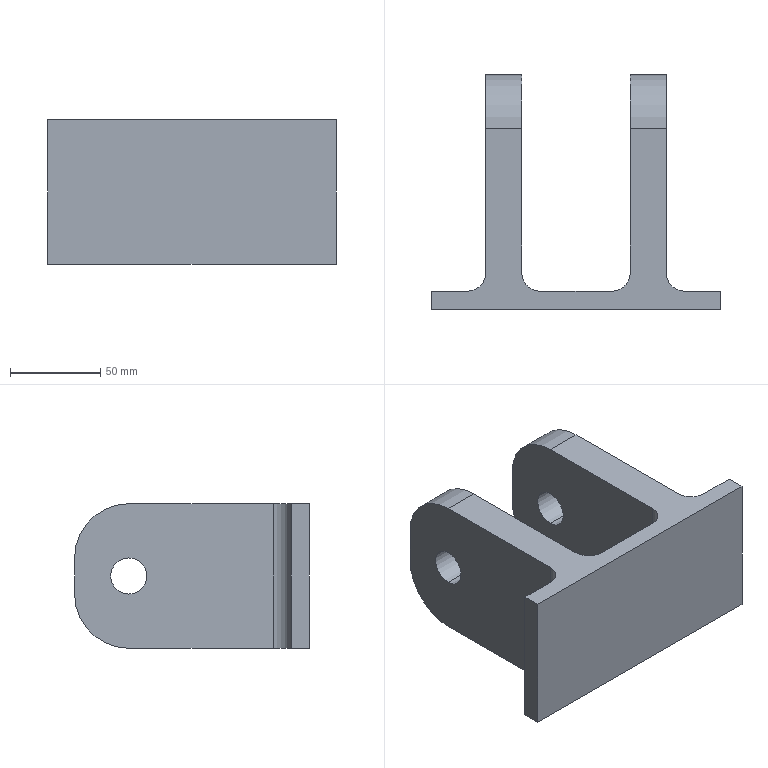Part | STEP file | Hydraulic cylinder base | 1 solid | 26 faces | box 160 x 130 x 80 mm | volume 490850 mm3 | plane 14 | cylinder 12 | commonest cylinder face diameters 20 x8 60 x4
STEP:
#1=CARTESIAN_POINT('',(50.,100.,10.));
#2=VERTEX_POINT('',#1);
#3=CARTESIAN_POINT('',(50.,100.,-10.));
#4=VERTEX_POINT('',#3);
#5=CARTESIAN_POINT('',(50.,100.,0.));
#6=DIRECTION('',(1.,0.,0.));
#7=DIRECTION('',(0.,0.,-1.));
#8=AXIS2_PLACEMENT_3D('',#5,#6,#7);
#9=CIRCLE('',#8,10.);
#10=EDGE_CURVE('',#2,#4,#9,.T.);
#11=ORIENTED_EDGE('',*,*,#10,.T.);
#12=CARTESIAN_POINT('',(30.,100.,-10.));
#13=VERTEX_POINT('',#12);
#14=CARTESIAN_POINT('',(80.001,100.,-10.));
#15=DIRECTION('',(-1.,0.,0.));
#16=VECTOR('',#15,1000.);
#17=LINE('',#14,#16);
#18=EDGE_CURVE('',#4,#13,#17,.T.);
#19=ORIENTED_EDGE('',*,*,#18,.T.);
#20=CARTESIAN_POINT('',(30.,100.,10.));
#21=VERTEX_POINT('',#20);
#22=CARTESIAN_POINT('',(30.,100.,0.));
#23=DIRECTION('',(1.,0.,0.));
#24=DIRECTION('',(0.,0.,-1.));
#25=AXIS2_PLACEMENT_3D('',#22,#23,#24);
#26=CIRCLE('',#25,10.);
#27=EDGE_CURVE('',#21,#13,#26,.T.);
#28=ORIENTED_EDGE('',*,*,#27,.F.);
#29=CARTESIAN_POINT('',(80.001,100.,10.));
#30=DIRECTION('',(-1.,0.,0.));
#31=VECTOR('',#30,1000.);
#32=LINE('',#29,#31);
#33=EDGE_CURVE('',#2,#21,#32,.T.);
#34=ORIENTED_EDGE('',*,*,#33,.F.);
#35=EDGE_LOOP('',(#11,#19,#28,#34));
#36=FACE_OUTER_BOUND('',#35,.T.);
#37=CARTESIAN_POINT('',(80.001,100.,0.));
#38=DIRECTION('',(-1.,0.,0.));
#39=DIRECTION('',(0.,0.,1.));
#40=AXIS2_PLACEMENT_3D('',#37,#38,#39);
#41=CYLINDRICAL_SURFACE('',#40,10.);
#42=ADVANCED_FACE('',(#36),#41,.F.);
#43=CARTESIAN_POINT('',(-50.,100.,-10.));
#44=VERTEX_POINT('',#43);
#45=CARTESIAN_POINT('',(-50.,100.,10.));
#46=VERTEX_POINT('',#45);
#47=CARTESIAN_POINT('',(-50.,100.,0.));
#48=DIRECTION('',(-1.,0.,0.));
#49=DIRECTION('',(0.,0.,-1.));
#50=AXIS2_PLACEMENT_3D('',#47,#48,#49);
#51=CIRCLE('',#50,10.);
#52=EDGE_CURVE('',#44,#46,#51,.T.);
#53=ORIENTED_EDGE('',*,*,#52,.T.);
#54=CARTESIAN_POINT('',(-30.,100.,10.));
#55=VERTEX_POINT('',#54);
#56=CARTESIAN_POINT('',(-80.001,100.,10.));
#57=DIRECTION('',(1.,0.,0.));
#58=VECTOR('',#57,1000.);
#59=LINE('',#56,#58);
#60=EDGE_CURVE('',#46,#55,#59,.T.);
#61=ORIENTED_EDGE('',*,*,#60,.T.);
#62=CARTESIAN_POINT('',(-30.,100.,-10.));
#63=VERTEX_POINT('',#62);
#64=CARTESIAN_POINT('',(-30.,100.,0.));
#65=DIRECTION('',(1.,0.,0.));
#66=DIRECTION('',(0.,0.,-1.));
#67=AXIS2_PLACEMENT_3D('',#64,#65,#66);
#68=CIRCLE('',#67,10.);
#69=EDGE_CURVE('',#55,#63,#68,.T.);
#70=ORIENTED_EDGE('',*,*,#69,.T.);
#71=CARTESIAN_POINT('',(-80.001,100.,-10.));
#72=DIRECTION('',(1.,0.,0.));
#73=VECTOR('',#72,1000.);
#74=LINE('',#71,#73);
#75=EDGE_CURVE('',#44,#63,#74,.T.);
#76=ORIENTED_EDGE('',*,*,#75,.F.);
#77=EDGE_LOOP('',(#53,#61,#70,#76));
#78=FACE_OUTER_BOUND('',#77,.T.);
#79=CARTESIAN_POINT('',(-80.001,100.,0.));
#80=DIRECTION('',(1.,0.,0.));
#81=DIRECTION('',(0.,0.,-1.));
#82=AXIS2_PLACEMENT_3D('',#79,#80,#81);
#83=CYLINDRICAL_SURFACE('',#82,10.);
#84=ADVANCED_FACE('',(#78),#83,.F.);
#85=CARTESIAN_POINT('',(80.,10.,-40.));
#86=VERTEX_POINT('',#85);
#87=CARTESIAN_POINT('',(60.,10.,-40.));
#88=VERTEX_POINT('',#87);
#89=CARTESIAN_POINT('',(-80.,10.,-40.));
#90=DIRECTION('',(-1.,0.,0.));
#91=VECTOR('',#90,1000.);
#92=LINE('',#89,#91);
#93=EDGE_CURVE('',#86,#88,#92,.T.);
#94=ORIENTED_EDGE('',*,*,#93,.T.);
#95=CARTESIAN_POINT('',(60.,10.,40.));
#96=VERTEX_POINT('',#95);
#97=CARTESIAN_POINT('',(60.,10.,40.));
#98=DIRECTION('',(0.,0.,1.));
#99=VECTOR('',#98,1000.);
#100=LINE('',#97,#99);
#101=EDGE_CURVE('',#88,#96,#100,.T.);
#102=ORIENTED_EDGE('',*,*,#101,.T.);
#103=CARTESIAN_POINT('',(80.,10.,40.));
#104=VERTEX_POINT('',#103);
#105=CARTESIAN_POINT('',(-80.,10.,40.));
#106=DIRECTION('',(1.,0.,0.));
#107=VECTOR('',#106,1000.);
#108=LINE('',#105,#107);
#109=EDGE_CURVE('',#96,#104,#108,.T.);
#110=ORIENTED_EDGE('',*,*,#109,.T.);
#111=CARTESIAN_POINT('',(80.,10.,-40.));
#112=DIRECTION('',(0.,0.,-1.));
#113=VECTOR('',#112,1000.);
#114=LINE('',#111,#113);
#115=EDGE_CURVE('',#104,#86,#114,.T.);
#116=ORIENTED_EDGE('',*,*,#115,.T.);
#117=EDGE_LOOP('',(#94,#102,#110,#116));
#118=FACE_OUTER_BOUND('',#117,.T.);
#119=CARTESIAN_POINT('',(0.,10.,0.));
#120=DIRECTION('',(0.,1.,0.));
#121=DIRECTION('',(0.,0.,1.));
#122=AXIS2_PLACEMENT_3D('',#119,#120,#121);
#123=PLANE('',#122);
#124=ADVANCED_FACE('',(#118),#123,.T.);
#125=CARTESIAN_POINT('',(-80.,10.,40.));
#126=VERTEX_POINT('',#125);
#127=CARTESIAN_POINT('',(-60.,10.,40.));
#128=VERTEX_POINT('',#127);
#129=CARTESIAN_POINT('',(-80.,10.,40.));
#130=DIRECTION('',(1.,0.,0.));
#131=VECTOR('',#130,1000.);
#132=LINE('',#129,#131);
#133=EDGE_CURVE('',#126,#128,#132,.T.);
#134=ORIENTED_EDGE('',*,*,#133,.T.);
#135=CARTESIAN_POINT('',(-60.,10.,-40.));
#136=VERTEX_POINT('',#135);
#137=CARTESIAN_POINT('',(-60.,10.,0.));
#138=DIRECTION('',(0.,0.,-1.));
#139=VECTOR('',#138,1000.);
#140=LINE('',#137,#139);
#141=EDGE_CURVE('',#128,#136,#140,.T.);
#142=ORIENTED_EDGE('',*,*,#141,.T.);
#143=CARTESIAN_POINT('',(-80.,10.,-40.));
#144=VERTEX_POINT('',#143);
#145=CARTESIAN_POINT('',(-80.,10.,-40.));
#146=DIRECTION('',(-1.,0.,0.));
#147=VECTOR('',#146,1000.);
#148=LINE('',#145,#147);
#149=EDGE_CURVE('',#136,#144,#148,.T.);
#150=ORIENTED_EDGE('',*,*,#149,.T.);
#151=CARTESIAN_POINT('',(-80.,10.,-40.));
#152=DIRECTION('',(0.,0.,1.));
#153=VECTOR('',#152,1000.);
#154=LINE('',#151,#153);
#155=EDGE_CURVE('',#144,#126,#154,.T.);
#156=ORIENTED_EDGE('',*,*,#155,.T.);
#157=EDGE_LOOP('',(#134,#142,#150,#156));
#158=FACE_OUTER_BOUND('',#157,.T.);
#159=CARTESIAN_POINT('',(0.,10.,0.));
#160=DIRECTION('',(0.,1.,0.));
#161=DIRECTION('',(0.,0.,1.));
#162=AXIS2_PLACEMENT_3D('',#159,#160,#161);
#163=PLANE('',#162);
#164=ADVANCED_FACE('',(#158),#163,.T.);
#165=CARTESIAN_POINT('',(80.,0.,40.));
#166=VERTEX_POINT('',#165);
#167=CARTESIAN_POINT('',(80.,0.,-40.));
#168=VERTEX_POINT('',#167);
#169=CARTESIAN_POINT('',(80.,0.,-40.));
#170=DIRECTION('',(0.,0.,-1.));
#171=VECTOR('',#170,1000.);
#172=LINE('',#169,#171);
#173=EDGE_CURVE('',#166,#168,#172,.T.);
#174=ORIENTED_EDGE('',*,*,#173,.T.);
#175=CARTESIAN_POINT('',(80.,10.,-40.));
#176=DIRECTION('',(0.,-1.,0.));
#177=VECTOR('',#176,1000.);
#178=LINE('',#175,#177);
#179=EDGE_CURVE('',#86,#168,#178,.T.);
#180=ORIENTED_EDGE('',*,*,#179,.F.);
#181=ORIENTED_EDGE('',*,*,#115,.F.);
#182=CARTESIAN_POINT('',(80.,10.,40.));
#183=DIRECTION('',(0.,-1.,0.));
#184=VECTOR('',#183,1000.);
#185=LINE('',#182,#184);
#186=EDGE_CURVE('',#104,#166,#185,.T.);
#187=ORIENTED_EDGE('',*,*,#186,.T.);
#188=EDGE_LOOP('',(#174,#180,#181,#187));
#189=FACE_OUTER_BOUND('',#188,.T.);
#190=CARTESIAN_POINT('',(80.,10.,-40.));
#191=DIRECTION('',(-1.,0.,0.));
#192=DIRECTION('',(0.,0.,1.));
#193=AXIS2_PLACEMENT_3D('',#190,#191,#192);
#194=PLANE('',#193);
#195=ADVANCED_FACE('',(#189),#194,.F.);
#196=CARTESIAN_POINT('',(30.,100.,-40.));
#197=VERTEX_POINT('',#196);
#198=CARTESIAN_POINT('',(30.,20.,-40.));
#199=VERTEX_POINT('',#198);
#200=CARTESIAN_POINT('',(30.,130.,-40.));
#201=DIRECTION('',(0.,-1.,0.));
#202=VECTOR('',#201,1000.);
#203=LINE('',#200,#202);
#204=EDGE_CURVE('',#197,#199,#203,.T.);
#205=ORIENTED_EDGE('',*,*,#204,.F.);
#206=CARTESIAN_POINT('',(50.,100.,-40.));
#207=VERTEX_POINT('',#206);
#208=CARTESIAN_POINT('',(50.,100.,-40.));
#209=DIRECTION('',(1.,0.,0.));
#210=VECTOR('',#209,1000.);
#211=LINE('',#208,#210);
#212=EDGE_CURVE('',#197,#207,#211,.T.);
#213=ORIENTED_EDGE('',*,*,#212,.T.);
#214=CARTESIAN_POINT('',(50.,20.,-40.));
#215=VERTEX_POINT('',#214);
#216=CARTESIAN_POINT('',(50.,130.,-40.));
#217=DIRECTION('',(0.,-1.,0.));
#218=VECTOR('',#217,1000.);
#219=LINE('',#216,#218);
#220=EDGE_CURVE('',#207,#215,#219,.T.);
#221=ORIENTED_EDGE('',*,*,#220,.T.);
#222=CARTESIAN_POINT('',(60.,20.,-40.));
#223=DIRECTION('',(0.,0.,1.));
#224=DIRECTION('',(1.,0.,0.));
#225=AXIS2_PLACEMENT_3D('',#222,#223,#224);
#226=CIRCLE('',#225,10.);
#227=EDGE_CURVE('',#215,#88,#226,.T.);
#228=ORIENTED_EDGE('',*,*,#227,.T.);
#229=ORIENTED_EDGE('',*,*,#93,.F.);
#230=ORIENTED_EDGE('',*,*,#179,.T.);
#231=CARTESIAN_POINT('',(-80.,0.,-40.));
#232=VERTEX_POINT('',#231);
#233=CARTESIAN_POINT('',(-80.,0.,-40.));
#234=DIRECTION('',(-1.,0.,0.));
#235=VECTOR('',#234,1000.);
#236=LINE('',#233,#235);
#237=EDGE_CURVE('',#168,#232,#236,.T.);
#238=ORIENTED_EDGE('',*,*,#237,.T.);
#239=CARTESIAN_POINT('',(-80.,10.,-40.));
#240=DIRECTION('',(0.,-1.,0.));
#241=VECTOR('',#240,1000.);
#242=LINE('',#239,#241);
#243=EDGE_CURVE('',#144,#232,#242,.T.);
#244=ORIENTED_EDGE('',*,*,#243,.F.);
#245=ORIENTED_EDGE('',*,*,#149,.F.);
#246=CARTESIAN_POINT('',(-50.,20.,-40.));
#247=VERTEX_POINT('',#246);
#248=CARTESIAN_POINT('',(-60.,20.,-40.));
#249=DIRECTION('',(0.,0.,1.));
#250=DIRECTION('',(1.,0.,0.));
#251=AXIS2_PLACEMENT_3D('',#248,#249,#250);
#252=CIRCLE('',#251,10.);
#253=EDGE_CURVE('',#136,#247,#252,.T.);
#254=ORIENTED_EDGE('',*,*,#253,.T.);
#255=CARTESIAN_POINT('',(-50.,100.,-40.));
#256=VERTEX_POINT('',#255);
#257=CARTESIAN_POINT('',(-50.,130.,-40.));
#258=DIRECTION('',(0.,-1.,0.));
#259=VECTOR('',#258,1000.);
#260=LINE('',#257,#259);
#261=EDGE_CURVE('',#256,#247,#260,.T.);
#262=ORIENTED_EDGE('',*,*,#261,.F.);
#263=CARTESIAN_POINT('',(-30.,100.,-40.));
#264=VERTEX_POINT('',#263);
#265=CARTESIAN_POINT('',(-30.,100.,-40.));
#266=DIRECTION('',(1.,0.,0.));
#267=VECTOR('',#266,1000.);
#268=LINE('',#265,#267);
#269=EDGE_CURVE('',#256,#264,#268,.T.);
#270=ORIENTED_EDGE('',*,*,#269,.T.);
#271=CARTESIAN_POINT('',(-30.,20.,-40.));
#272=VERTEX_POINT('',#271);
#273=CARTESIAN_POINT('',(-30.,130.,-40.));
#274=DIRECTION('',(0.,-1.,0.));
#275=VECTOR('',#274,1000.);
#276=LINE('',#273,#275);
#277=EDGE_CURVE('',#264,#272,#276,.T.);
#278=ORIENTED_EDGE('',*,*,#277,.T.);
#279=CARTESIAN_POINT('',(-20.,10.,-40.));
#280=VERTEX_POINT('',#279);
#281=CARTESIAN_POINT('',(-20.,20.,-40.));
#282=DIRECTION('',(0.,0.,1.));
#283=DIRECTION('',(1.,0.,0.));
#284=AXIS2_PLACEMENT_3D('',#281,#282,#283);
#285=CIRCLE('',#284,10.);
#286=EDGE_CURVE('',#272,#280,#285,.T.);
#287=ORIENTED_EDGE('',*,*,#286,.T.);
#288=CARTESIAN_POINT('',(20.,10.,-40.));
#289=VERTEX_POINT('',#288);
#290=CARTESIAN_POINT('',(-80.,10.,-40.));
#291=DIRECTION('',(-1.,0.,0.));
#292=VECTOR('',#291,1000.);
#293=LINE('',#290,#292);
#294=EDGE_CURVE('',#289,#280,#293,.T.);
#295=ORIENTED_EDGE('',*,*,#294,.F.);
#296=CARTESIAN_POINT('',(20.,20.,-40.));
#297=DIRECTION('',(0.,0.,1.));
#298=DIRECTION('',(1.,0.,0.));
#299=AXIS2_PLACEMENT_3D('',#296,#297,#298);
#300=CIRCLE('',#299,10.);
#301=EDGE_CURVE('',#289,#199,#300,.T.);
#302=ORIENTED_EDGE('',*,*,#301,.T.);
#303=EDGE_LOOP('',(#205,#213,#221,#228,#229,#230,#238,#244,#245,#254,#262,#270,#278,#287,#295,#302));
#304=FACE_OUTER_BOUND('',#303,.T.);
#305=CARTESIAN_POINT('',(-80.,10.,-40.));
#306=DIRECTION('',(0.,0.,1.));
#307=DIRECTION('',(1.,0.,0.));
#308=AXIS2_PLACEMENT_3D('',#305,#306,#307);
#309=PLANE('',#308);
#310=ADVANCED_FACE('',(#304),#309,.F.);
#311=CARTESIAN_POINT('',(-80.,0.,40.));
#312=VERTEX_POINT('',#311);
#313=CARTESIAN_POINT('',(-80.,0.,-40.));
#314=DIRECTION('',(0.,0.,1.));
#315=VECTOR('',#314,1000.);
#316=LINE('',#313,#315);
#317=EDGE_CURVE('',#232,#312,#316,.T.);
#318=ORIENTED_EDGE('',*,*,#317,.T.);
#319=CARTESIAN_POINT('',(-80.,10.,40.));
#320=DIRECTION('',(0.,-1.,0.));
#321=VECTOR('',#320,1000.);
#322=LINE('',#319,#321);
#323=EDGE_CURVE('',#126,#312,#322,.T.);
#324=ORIENTED_EDGE('',*,*,#323,.F.);
#325=ORIENTED_EDGE('',*,*,#155,.F.);
#326=ORIENTED_EDGE('',*,*,#243,.T.);
#327=EDGE_LOOP('',(#318,#324,#325,#326));
#328=FACE_OUTER_BOUND('',#327,.T.);
#329=CARTESIAN_POINT('',(-80.,10.,-40.));
#330=DIRECTION('',(1.,0.,0.));
#331=DIRECTION('',(0.,0.,-1.));
#332=AXIS2_PLACEMENT_3D('',#329,#330,#331);
#333=PLANE('',#332);
#334=ADVANCED_FACE('',(#328),#333,.F.);
#335=CARTESIAN_POINT('',(50.,100.,40.));
#336=VERTEX_POINT('',#335);
#337=CARTESIAN_POINT('',(50.,20.,40.));
#338=VERTEX_POINT('',#337);
#339=CARTESIAN_POINT('',(50.,130.,40.));
#340=DIRECTION('',(0.,-1.,0.));
#341=VECTOR('',#340,1000.);
#342=LINE('',#339,#341);
#343=EDGE_CURVE('',#336,#338,#342,.T.);
#344=ORIENTED_EDGE('',*,*,#343,.F.);
#345=CARTESIAN_POINT('',(30.,100.,40.));
#346=VERTEX_POINT('',#345);
#347=CARTESIAN_POINT('',(30.,100.,40.));
#348=DIRECTION('',(-1.,0.,0.));
#349=VECTOR('',#348,1000.);
#350=LINE('',#347,#349);
#351=EDGE_CURVE('',#336,#346,#350,.T.);
#352=ORIENTED_EDGE('',*,*,#351,.T.);
#353=CARTESIAN_POINT('',(30.,20.,40.));
#354=VERTEX_POINT('',#353);
#355=CARTESIAN_POINT('',(30.,130.,40.));
#356=DIRECTION('',(0.,-1.,0.));
#357=VECTOR('',#356,1000.);
#358=LINE('',#355,#357);
#359=EDGE_CURVE('',#346,#354,#358,.T.);
#360=ORIENTED_EDGE('',*,*,#359,.T.);
#361=CARTESIAN_POINT('',(20.,10.,40.));
#362=VERTEX_POINT('',#361);
#363=CARTESIAN_POINT('',(20.,20.,40.));
#364=DIRECTION('',(0.,0.,-1.));
#365=DIRECTION('',(-1.,0.,0.));
#366=AXIS2_PLACEMENT_3D('',#363,#364,#365);
#367=CIRCLE('',#366,10.);
#368=EDGE_CURVE('',#354,#362,#367,.T.);
#369=ORIENTED_EDGE('',*,*,#368,.T.);
#370=CARTESIAN_POINT('',(-20.,10.,40.));
#371=VERTEX_POINT('',#370);
#372=CARTESIAN_POINT('',(-80.,10.,40.));
#373=DIRECTION('',(1.,0.,0.));
#374=VECTOR('',#373,1000.);
#375=LINE('',#372,#374);
#376=EDGE_CURVE('',#371,#362,#375,.T.);
#377=ORIENTED_EDGE('',*,*,#376,.F.);
#378=CARTESIAN_POINT('',(-30.,20.,40.));
#379=VERTEX_POINT('',#378);
#380=CARTESIAN_POINT('',(-20.,20.,40.));
#381=DIRECTION('',(0.,0.,-1.));
#382=DIRECTION('',(-1.,0.,0.));
#383=AXIS2_PLACEMENT_3D('',#380,#381,#382);
#384=CIRCLE('',#383,10.);
#385=EDGE_CURVE('',#371,#379,#384,.T.);
#386=ORIENTED_EDGE('',*,*,#385,.T.);
#387=CARTESIAN_POINT('',(-30.,100.,40.));
#388=VERTEX_POINT('',#387);
#389=CARTESIAN_POINT('',(-30.,130.,40.));
#390=DIRECTION('',(0.,-1.,0.));
#391=VECTOR('',#390,1000.);
#392=LINE('',#389,#391);
#393=EDGE_CURVE('',#388,#379,#392,.T.);
#394=ORIENTED_EDGE('',*,*,#393,.F.);
#395=CARTESIAN_POINT('',(-50.,100.,40.));
#396=VERTEX_POINT('',#395);
#397=CARTESIAN_POINT('',(-50.,100.,40.));
#398=DIRECTION('',(-1.,0.,0.));
#399=VECTOR('',#398,1000.);
#400=LINE('',#397,#399);
#401=EDGE_CURVE('',#388,#396,#400,.T.);
#402=ORIENTED_EDGE('',*,*,#401,.T.);
#403=CARTESIAN_POINT('',(-50.,20.,40.));
#404=VERTEX_POINT('',#403);
#405=CARTESIAN_POINT('',(-50.,130.,40.));
#406=DIRECTION('',(0.,-1.,0.));
#407=VECTOR('',#406,1000.);
#408=LINE('',#405,#407);
#409=EDGE_CURVE('',#396,#404,#408,.T.);
#410=ORIENTED_EDGE('',*,*,#409,.T.);
#411=CARTESIAN_POINT('',(-60.,20.,40.));
#412=DIRECTION('',(0.,0.,-1.));
#413=DIRECTION('',(-1.,0.,0.));
#414=AXIS2_PLACEMENT_3D('',#411,#412,#413);
#415=CIRCLE('',#414,10.);
#416=EDGE_CURVE('',#404,#128,#415,.T.);
#417=ORIENTED_EDGE('',*,*,#416,.T.);
#418=ORIENTED_EDGE('',*,*,#133,.F.);
#419=ORIENTED_EDGE('',*,*,#323,.T.);
#420=CARTESIAN_POINT('',(-80.,0.,40.));
#421=DIRECTION('',(1.,0.,0.));
#422=VECTOR('',#421,1000.);
#423=LINE('',#420,#422);
#424=EDGE_CURVE('',#312,#166,#423,.T.);
#425=ORIENTED_EDGE('',*,*,#424,.T.);
#426=ORIENTED_EDGE('',*,*,#186,.F.);
#427=ORIENTED_EDGE('',*,*,#109,.F.);
#428=CARTESIAN_POINT('',(60.,20.,40.));
#429=DIRECTION('',(0.,0.,-1.));
#430=DIRECTION('',(-1.,0.,0.));
#431=AXIS2_PLACEMENT_3D('',#428,#429,#430);
#432=CIRCLE('',#431,10.);
#433=EDGE_CURVE('',#96,#338,#432,.T.);
#434=ORIENTED_EDGE('',*,*,#433,.T.);
#435=EDGE_LOOP('',(#344,#352,#360,#369,#377,#386,#394,#402,#410,#417,#418,#419,#425,#426,#427,#434));
#436=FACE_OUTER_BOUND('',#435,.T.);
#437=CARTESIAN_POINT('',(-80.,10.,40.));
#438=DIRECTION('',(0.,0.,-1.));
#439=DIRECTION('',(-1.,0.,0.));
#440=AXIS2_PLACEMENT_3D('',#437,#438,#439);
#441=PLANE('',#440);
#442=ADVANCED_FACE('',(#436),#441,.F.);
#443=ORIENTED_EDGE('',*,*,#376,.T.);
#444=CARTESIAN_POINT('',(20.,10.,-40.));
#445=DIRECTION('',(0.,0.,-1.));
#446=VECTOR('',#445,1000.);
#447=LINE('',#444,#446);
#448=EDGE_CURVE('',#362,#289,#447,.T.);
#449=ORIENTED_EDGE('',*,*,#448,.T.);
#450=ORIENTED_EDGE('',*,*,#294,.T.);
#451=CARTESIAN_POINT('',(-20.,10.,0.));
#452=DIRECTION('',(0.,0.,1.));
#453=VECTOR('',#452,1000.);
#454=LINE('',#451,#453);
#455=EDGE_CURVE('',#280,#371,#454,.T.);
#456=ORIENTED_EDGE('',*,*,#455,.T.);
#457=EDGE_LOOP('',(#443,#449,#450,#456));
#458=FACE_OUTER_BOUND('',#457,.T.);
#459=CARTESIAN_POINT('',(0.,10.,0.));
#460=DIRECTION('',(0.,1.,0.));
#461=DIRECTION('',(0.,0.,1.));
#462=AXIS2_PLACEMENT_3D('',#459,#460,#461);
#463=PLANE('',#462);
#464=ADVANCED_FACE('',(#458),#463,.T.);
#465=ORIENTED_EDGE('',*,*,#173,.F.);
#466=ORIENTED_EDGE('',*,*,#424,.F.);
#467=ORIENTED_EDGE('',*,*,#317,.F.);
#468=ORIENTED_EDGE('',*,*,#237,.F.);
#469=EDGE_LOOP('',(#465,#466,#467,#468));
#470=FACE_OUTER_BOUND('',#469,.T.);
#471=CARTESIAN_POINT('',(0.,0.,0.));
#472=DIRECTION('',(0.,1.,0.));
#473=DIRECTION('',(0.,0.,1.));
#474=AXIS2_PLACEMENT_3D('',#471,#472,#473);
#475=PLANE('',#474);
#476=ADVANCED_FACE('',(#470),#475,.F.);
#477=ORIENTED_EDGE('',*,*,#52,.F.);
#478=CARTESIAN_POINT('',(-50.,100.,0.));
#479=DIRECTION('',(-1.,0.,0.));
#480=DIRECTION('',(0.,0.,-1.));
#481=AXIS2_PLACEMENT_3D('',#478,#479,#480);
#482=CIRCLE('',#481,10.);
#483=EDGE_CURVE('',#46,#44,#482,.T.);
#484=ORIENTED_EDGE('',*,*,#483,.F.);
#485=EDGE_LOOP('',(#477,#484));
#486=FACE_BOUND('',#485,.T.);
#487=CARTESIAN_POINT('',(-50.,130.,-10.));
#488=VERTEX_POINT('',#487);
#489=CARTESIAN_POINT('',(-50.,130.,10.));
#490=VERTEX_POINT('',#489);
#491=CARTESIAN_POINT('',(-50.,130.,-40.));
#492=DIRECTION('',(0.,0.,1.));
#493=VECTOR('',#492,1000.);
#494=LINE('',#491,#493);
#495=EDGE_CURVE('',#488,#490,#494,.T.);
#496=ORIENTED_EDGE('',*,*,#495,.F.);
#497=CARTESIAN_POINT('',(-50.,100.,-10.));
#498=DIRECTION('',(-1.,0.,0.));
#499=DIRECTION('',(0.,0.,-1.));
#500=AXIS2_PLACEMENT_3D('',#497,#498,#499);
#501=CIRCLE('',#500,30.);
#502=EDGE_CURVE('',#488,#256,#501,.T.);
#503=ORIENTED_EDGE('',*,*,#502,.T.);
#504=ORIENTED_EDGE('',*,*,#261,.T.);
#505=CARTESIAN_POINT('',(-50.,20.,-40.));
#506=DIRECTION('',(0.,0.,1.));
#507=VECTOR('',#506,1000.);
#508=LINE('',#505,#507);
#509=EDGE_CURVE('',#247,#404,#508,.T.);
#510=ORIENTED_EDGE('',*,*,#509,.T.);
#511=ORIENTED_EDGE('',*,*,#409,.F.);
#512=CARTESIAN_POINT('',(-50.,100.,10.));
#513=DIRECTION('',(-1.,0.,0.));
#514=DIRECTION('',(0.,0.,-1.));
#515=AXIS2_PLACEMENT_3D('',#512,#513,#514);
#516=CIRCLE('',#515,30.);
#517=EDGE_CURVE('',#396,#490,#516,.T.);
#518=ORIENTED_EDGE('',*,*,#517,.T.);
#519=EDGE_LOOP('',(#496,#503,#504,#510,#511,#518));
#520=FACE_OUTER_BOUND('',#519,.T.);
#521=CARTESIAN_POINT('',(-50.,130.,-40.));
#522=DIRECTION('',(1.,0.,0.));
#523=DIRECTION('',(0.,0.,-1.));
#524=AXIS2_PLACEMENT_3D('',#521,#522,#523);
#525=PLANE('',#524);
#526=ADVANCED_FACE('',(#486,#520),#525,.F.);
#527=CARTESIAN_POINT('',(-30.,100.,0.));
#528=DIRECTION('',(1.,0.,0.));
#529=DIRECTION('',(0.,0.,-1.));
#530=AXIS2_PLACEMENT_3D('',#527,#528,#529);
#531=CIRCLE('',#530,10.);
#532=EDGE_CURVE('',#63,#55,#531,.T.);
#533=ORIENTED_EDGE('',*,*,#532,.F.);
#534=ORIENTED_EDGE('',*,*,#69,.F.);
#535=EDGE_LOOP('',(#533,#534));
#536=FACE_BOUND('',#535,.T.);
#537=ORIENTED_EDGE('',*,*,#277,.F.);
#538=CARTESIAN_POINT('',(-30.,130.,-10.));
#539=VERTEX_POINT('',#538);
#540=CARTESIAN_POINT('',(-30.,100.,-10.));
#541=DIRECTION('',(1.,0.,0.));
#542=DIRECTION('',(0.,0.,1.));
#543=AXIS2_PLACEMENT_3D('',#540,#541,#542);
#544=CIRCLE('',#543,30.);
#545=EDGE_CURVE('',#264,#539,#544,.T.);
#546=ORIENTED_EDGE('',*,*,#545,.T.);
#547=CARTESIAN_POINT('',(-30.,130.,10.));
#548=VERTEX_POINT('',#547);
#549=CARTESIAN_POINT('',(-30.,130.,-40.));
#550=DIRECTION('',(0.,0.,-1.));
#551=VECTOR('',#550,1000.);
#552=LINE('',#549,#551);
#553=EDGE_CURVE('',#548,#539,#552,.T.);
#554=ORIENTED_EDGE('',*,*,#553,.F.);
#555=CARTESIAN_POINT('',(-30.,100.,10.));
#556=DIRECTION('',(1.,0.,0.));
#557=DIRECTION('',(0.,0.,1.));
#558=AXIS2_PLACEMENT_3D('',#555,#556,#557);
#559=CIRCLE('',#558,30.);
#560=EDGE_CURVE('',#548,#388,#559,.T.);
#561=ORIENTED_EDGE('',*,*,#560,.T.);
#562=ORIENTED_EDGE('',*,*,#393,.T.);
#563=CARTESIAN_POINT('',(-30.,20.,-40.));
#564=DIRECTION('',(0.,0.,-1.));
#565=VECTOR('',#564,1000.);
#566=LINE('',#563,#565);
#567=EDGE_CURVE('',#379,#272,#566,.T.);
#568=ORIENTED_EDGE('',*,*,#567,.T.);
#569=EDGE_LOOP('',(#537,#546,#554,#561,#562,#568));
#570=FACE_OUTER_BOUND('',#569,.T.);
#571=CARTESIAN_POINT('',(-30.,130.,-40.));
#572=DIRECTION('',(-1.,0.,0.));
#573=DIRECTION('',(0.,0.,1.));
#574=AXIS2_PLACEMENT_3D('',#571,#572,#573);
#575=PLANE('',#574);
#576=ADVANCED_FACE('',(#536,#570),#575,.F.);
#577=ORIENTED_EDGE('',*,*,#553,.T.);
#578=CARTESIAN_POINT('',(-50.,130.,-10.));
#579=DIRECTION('',(-1.,0.,0.));
#580=VECTOR('',#579,1000.);
#581=LINE('',#578,#580);
#582=EDGE_CURVE('',#539,#488,#581,.T.);
#583=ORIENTED_EDGE('',*,*,#582,.T.);
#584=ORIENTED_EDGE('',*,*,#495,.T.);
#585=CARTESIAN_POINT('',(-30.,130.,10.));
#586=DIRECTION('',(1.,0.,0.));
#587=VECTOR('',#586,1000.);
#588=LINE('',#585,#587);
#589=EDGE_CURVE('',#490,#548,#588,.T.);
#590=ORIENTED_EDGE('',*,*,#589,.T.);
#591=EDGE_LOOP('',(#577,#583,#584,#590));
#592=FACE_OUTER_BOUND('',#591,.T.);
#593=CARTESIAN_POINT('',(0.,130.,0.));
#594=DIRECTION('',(0.,1.,0.));
#595=DIRECTION('',(0.,0.,1.));
#596=AXIS2_PLACEMENT_3D('',#593,#594,#595);
#597=PLANE('',#596);
#598=ADVANCED_FACE('',(#592),#597,.T.);
#599=ORIENTED_EDGE('',*,*,#385,.F.);
#600=ORIENTED_EDGE('',*,*,#455,.F.);
#601=ORIENTED_EDGE('',*,*,#286,.F.);
#602=ORIENTED_EDGE('',*,*,#567,.F.);
#603=EDGE_LOOP('',(#599,#600,#601,#602));
#604=FACE_OUTER_BOUND('',#603,.T.);
#605=CARTESIAN_POINT('',(-20.,20.,-40.));
#606=DIRECTION('',(0.,0.,-1.));
#607=DIRECTION('',(-1.,0.,0.));
#608=AXIS2_PLACEMENT_3D('',#605,#606,#607);
#609=CYLINDRICAL_SURFACE('',#608,10.);
#610=ADVANCED_FACE('',(#604),#609,.F.);
#611=ORIENTED_EDGE('',*,*,#253,.F.);
#612=ORIENTED_EDGE('',*,*,#141,.F.);
#613=ORIENTED_EDGE('',*,*,#416,.F.);
#614=ORIENTED_EDGE('',*,*,#509,.F.);
#615=EDGE_LOOP('',(#611,#612,#613,#614));
#616=FACE_OUTER_BOUND('',#615,.T.);
#617=CARTESIAN_POINT('',(-60.,20.,-40.));
#618=DIRECTION('',(0.,0.,1.));
#619=DIRECTION('',(1.,0.,0.));
#620=AXIS2_PLACEMENT_3D('',#617,#618,#619);
#621=CYLINDRICAL_SURFACE('',#620,10.);
#622=ADVANCED_FACE('',(#616),#621,.F.);
#623=ORIENTED_EDGE('',*,*,#545,.F.);
#624=ORIENTED_EDGE('',*,*,#269,.F.);
#625=ORIENTED_EDGE('',*,*,#502,.F.);
#626=ORIENTED_EDGE('',*,*,#582,.F.);
#627=EDGE_LOOP('',(#623,#624,#625,#626));
#628=FACE_OUTER_BOUND('',#627,.T.);
#629=CARTESIAN_POINT('',(0.,100.,-10.));
#630=DIRECTION('',(1.,0.,0.));
#631=DIRECTION('',(0.,0.,-1.));
#632=AXIS2_PLACEMENT_3D('',#629,#630,#631);
#633=CYLINDRICAL_SURFACE('',#632,30.);
#634=ADVANCED_FACE('',(#628),#633,.T.);
#635=ORIENTED_EDGE('',*,*,#517,.F.);
#636=ORIENTED_EDGE('',*,*,#401,.F.);
#637=ORIENTED_EDGE('',*,*,#560,.F.);
#638=ORIENTED_EDGE('',*,*,#589,.F.);
#639=EDGE_LOOP('',(#635,#636,#637,#638));
#640=FACE_OUTER_BOUND('',#639,.T.);
#641=CARTESIAN_POINT('',(0.,100.,10.));
#642=DIRECTION('',(-1.,0.,0.));
#643=DIRECTION('',(0.,0.,1.));
#644=AXIS2_PLACEMENT_3D('',#641,#642,#643);
#645=CYLINDRICAL_SURFACE('',#644,30.);
#646=ADVANCED_FACE('',(#640),#645,.T.);
#647=ORIENTED_EDGE('',*,*,#60,.F.);
#648=ORIENTED_EDGE('',*,*,#483,.T.);
#649=ORIENTED_EDGE('',*,*,#75,.T.);
#650=ORIENTED_EDGE('',*,*,#532,.T.);
#651=EDGE_LOOP('',(#647,#648,#649,#650));
#652=FACE_OUTER_BOUND('',#651,.T.);
#653=CARTESIAN_POINT('',(-80.001,100.,0.));
#654=DIRECTION('',(1.,0.,0.));
#655=DIRECTION('',(0.,0.,-1.));
#656=AXIS2_PLACEMENT_3D('',#653,#654,#655);
#657=CYLINDRICAL_SURFACE('',#656,10.);
#658=ADVANCED_FACE('',(#652),#657,.F.);
#659=ORIENTED_EDGE('',*,*,#10,.F.);
#660=CARTESIAN_POINT('',(50.,100.,0.));
#661=DIRECTION('',(1.,0.,0.));
#662=DIRECTION('',(0.,0.,-1.));
#663=AXIS2_PLACEMENT_3D('',#660,#661,#662);
#664=CIRCLE('',#663,10.);
#665=EDGE_CURVE('',#4,#2,#664,.T.);
#666=ORIENTED_EDGE('',*,*,#665,.F.);
#667=EDGE_LOOP('',(#659,#666));
#668=FACE_BOUND('',#667,.T.);
#669=ORIENTED_EDGE('',*,*,#220,.F.);
#670=CARTESIAN_POINT('',(50.,130.,-10.));
#671=VERTEX_POINT('',#670);
#672=CARTESIAN_POINT('',(50.,100.,-10.));
#673=DIRECTION('',(1.,0.,0.));
#674=DIRECTION('',(0.,0.,-1.));
#675=AXIS2_PLACEMENT_3D('',#672,#673,#674);
#676=CIRCLE('',#675,30.);
#677=EDGE_CURVE('',#207,#671,#676,.T.);
#678=ORIENTED_EDGE('',*,*,#677,.T.);
#679=CARTESIAN_POINT('',(50.,130.,10.));
#680=VERTEX_POINT('',#679);
#681=CARTESIAN_POINT('',(50.,130.,-40.));
#682=DIRECTION('',(0.,0.,1.));
#683=VECTOR('',#682,1000.);
#684=LINE('',#681,#683);
#685=EDGE_CURVE('',#671,#680,#684,.T.);
#686=ORIENTED_EDGE('',*,*,#685,.T.);
#687=CARTESIAN_POINT('',(50.,100.,10.));
#688=DIRECTION('',(1.,0.,0.));
#689=DIRECTION('',(0.,0.,-1.));
#690=AXIS2_PLACEMENT_3D('',#687,#688,#689);
#691=CIRCLE('',#690,30.);
#692=EDGE_CURVE('',#680,#336,#691,.T.);
#693=ORIENTED_EDGE('',*,*,#692,.T.);
#694=ORIENTED_EDGE('',*,*,#343,.T.);
#695=CARTESIAN_POINT('',(50.,20.,-40.));
#696=DIRECTION('',(0.,0.,-1.));
#697=VECTOR('',#696,1000.);
#698=LINE('',#695,#697);
#699=EDGE_CURVE('',#338,#215,#698,.T.);
#700=ORIENTED_EDGE('',*,*,#699,.T.);
#701=EDGE_LOOP('',(#669,#678,#686,#693,#694,#700));
#702=FACE_OUTER_BOUND('',#701,.T.);
#703=CARTESIAN_POINT('',(50.,130.,-40.));
#704=DIRECTION('',(1.,0.,0.));
#705=DIRECTION('',(0.,0.,-1.));
#706=AXIS2_PLACEMENT_3D('',#703,#704,#705);
#707=PLANE('',#706);
#708=ADVANCED_FACE('',(#668,#702),#707,.T.);
#709=ORIENTED_EDGE('',*,*,#27,.T.);
#710=CARTESIAN_POINT('',(30.,100.,0.));
#711=DIRECTION('',(1.,0.,0.));
#712=DIRECTION('',(0.,0.,-1.));
#713=AXIS2_PLACEMENT_3D('',#710,#711,#712);
#714=CIRCLE('',#713,10.);
#715=EDGE_CURVE('',#13,#21,#714,.T.);
#716=ORIENTED_EDGE('',*,*,#715,.T.);
#717=EDGE_LOOP('',(#709,#716));
#718=FACE_BOUND('',#717,.T.);
#719=CARTESIAN_POINT('',(30.,130.,10.));
#720=VERTEX_POINT('',#719);
#721=CARTESIAN_POINT('',(30.,130.,-10.));
#722=VERTEX_POINT('',#721);
#723=CARTESIAN_POINT('',(30.,130.,-40.));
#724=DIRECTION('',(0.,0.,-1.));
#725=VECTOR('',#724,1000.);
#726=LINE('',#723,#725);
#727=EDGE_CURVE('',#720,#722,#726,.T.);
#728=ORIENTED_EDGE('',*,*,#727,.T.);
#729=CARTESIAN_POINT('',(30.,100.,-10.));
#730=DIRECTION('',(-1.,0.,0.));
#731=DIRECTION('',(0.,0.,1.));
#732=AXIS2_PLACEMENT_3D('',#729,#730,#731);
#733=CIRCLE('',#732,30.);
#734=EDGE_CURVE('',#722,#197,#733,.T.);
#735=ORIENTED_EDGE('',*,*,#734,.T.);
#736=ORIENTED_EDGE('',*,*,#204,.T.);
#737=CARTESIAN_POINT('',(30.,20.,40.));
#738=DIRECTION('',(0.,0.,1.));
#739=VECTOR('',#738,1000.);
#740=LINE('',#737,#739);
#741=EDGE_CURVE('',#199,#354,#740,.T.);
#742=ORIENTED_EDGE('',*,*,#741,.T.);
#743=ORIENTED_EDGE('',*,*,#359,.F.);
#744=CARTESIAN_POINT('',(30.,100.,10.));
#745=DIRECTION('',(-1.,0.,0.));
#746=DIRECTION('',(0.,0.,1.));
#747=AXIS2_PLACEMENT_3D('',#744,#745,#746);
#748=CIRCLE('',#747,30.);
#749=EDGE_CURVE('',#346,#720,#748,.T.);
#750=ORIENTED_EDGE('',*,*,#749,.T.);
#751=EDGE_LOOP('',(#728,#735,#736,#742,#743,#750));
#752=FACE_OUTER_BOUND('',#751,.T.);
#753=CARTESIAN_POINT('',(30.,130.,-40.));
#754=DIRECTION('',(-1.,0.,0.));
#755=DIRECTION('',(0.,0.,1.));
#756=AXIS2_PLACEMENT_3D('',#753,#754,#755);
#757=PLANE('',#756);
#758=ADVANCED_FACE('',(#718,#752),#757,.T.);
#759=ORIENTED_EDGE('',*,*,#685,.F.);
#760=CARTESIAN_POINT('',(30.,130.,-10.));
#761=DIRECTION('',(-1.,0.,0.));
#762=VECTOR('',#761,1000.);
#763=LINE('',#760,#762);
#764=EDGE_CURVE('',#671,#722,#763,.T.);
#765=ORIENTED_EDGE('',*,*,#764,.T.);
#766=ORIENTED_EDGE('',*,*,#727,.F.);
#767=CARTESIAN_POINT('',(50.,130.,10.));
#768=DIRECTION('',(1.,0.,0.));
#769=VECTOR('',#768,1000.);
#770=LINE('',#767,#769);
#771=EDGE_CURVE('',#720,#680,#770,.T.);
#772=ORIENTED_EDGE('',*,*,#771,.T.);
#773=EDGE_LOOP('',(#759,#765,#766,#772));
#774=FACE_OUTER_BOUND('',#773,.T.);
#775=CARTESIAN_POINT('',(0.,130.,0.));
#776=DIRECTION('',(0.,1.,0.));
#777=DIRECTION('',(0.,0.,1.));
#778=AXIS2_PLACEMENT_3D('',#775,#776,#777);
#779=PLANE('',#778);
#780=ADVANCED_FACE('',(#774),#779,.T.);
#781=ORIENTED_EDGE('',*,*,#368,.F.);
#782=ORIENTED_EDGE('',*,*,#741,.F.);
#783=ORIENTED_EDGE('',*,*,#301,.F.);
#784=ORIENTED_EDGE('',*,*,#448,.F.);
#785=EDGE_LOOP('',(#781,#782,#783,#784));
#786=FACE_OUTER_BOUND('',#785,.T.);
#787=CARTESIAN_POINT('',(20.,20.,0.));
#788=DIRECTION('',(0.,0.,1.));
#789=DIRECTION('',(1.,0.,0.));
#790=AXIS2_PLACEMENT_3D('',#787,#788,#789);
#791=CYLINDRICAL_SURFACE('',#790,10.);
#792=ADVANCED_FACE('',(#786),#791,.F.);
#793=ORIENTED_EDGE('',*,*,#227,.F.);
#794=ORIENTED_EDGE('',*,*,#699,.F.);
#795=ORIENTED_EDGE('',*,*,#433,.F.);
#796=ORIENTED_EDGE('',*,*,#101,.F.);
#797=EDGE_LOOP('',(#793,#794,#795,#796));
#798=FACE_OUTER_BOUND('',#797,.T.);
#799=CARTESIAN_POINT('',(60.,20.,0.));
#800=DIRECTION('',(0.,0.,-1.));
#801=DIRECTION('',(-1.,0.,0.));
#802=AXIS2_PLACEMENT_3D('',#799,#800,#801);
#803=CYLINDRICAL_SURFACE('',#802,10.);
#804=ADVANCED_FACE('',(#798),#803,.F.);
#805=ORIENTED_EDGE('',*,*,#734,.F.);
#806=ORIENTED_EDGE('',*,*,#764,.F.);
#807=ORIENTED_EDGE('',*,*,#677,.F.);
#808=ORIENTED_EDGE('',*,*,#212,.F.);
#809=EDGE_LOOP('',(#805,#806,#807,#808));
#810=FACE_OUTER_BOUND('',#809,.T.);
#811=CARTESIAN_POINT('',(-80.,100.,-10.));
#812=DIRECTION('',(-1.,0.,0.));
#813=DIRECTION('',(0.,0.,1.));
#814=AXIS2_PLACEMENT_3D('',#811,#812,#813);
#815=CYLINDRICAL_SURFACE('',#814,30.);
#816=ADVANCED_FACE('',(#810),#815,.T.);
#817=ORIENTED_EDGE('',*,*,#692,.F.);
#818=ORIENTED_EDGE('',*,*,#771,.F.);
#819=ORIENTED_EDGE('',*,*,#749,.F.);
#820=ORIENTED_EDGE('',*,*,#351,.F.);
#821=EDGE_LOOP('',(#817,#818,#819,#820));
#822=FACE_OUTER_BOUND('',#821,.T.);
#823=CARTESIAN_POINT('',(-80.,100.,10.));
#824=DIRECTION('',(1.,0.,0.));
#825=DIRECTION('',(0.,0.,-1.));
#826=AXIS2_PLACEMENT_3D('',#823,#824,#825);
#827=CYLINDRICAL_SURFACE('',#826,30.);
#828=ADVANCED_FACE('',(#822),#827,.T.);
#829=ORIENTED_EDGE('',*,*,#18,.F.);
#830=ORIENTED_EDGE('',*,*,#665,.T.);
#831=ORIENTED_EDGE('',*,*,#33,.T.);
#832=ORIENTED_EDGE('',*,*,#715,.F.);
#833=EDGE_LOOP('',(#829,#830,#831,#832));
#834=FACE_OUTER_BOUND('',#833,.T.);
#835=CARTESIAN_POINT('',(80.001,100.,0.));
#836=DIRECTION('',(-1.,0.,0.));
#837=DIRECTION('',(0.,0.,1.));
#838=AXIS2_PLACEMENT_3D('',#835,#836,#837);
#839=CYLINDRICAL_SURFACE('',#838,10.);
#840=ADVANCED_FACE('',(#834),#839,.F.);
#841=CLOSED_SHELL('',(#42,#84,#124,#164,#195,#310,#334,#442,#464,#476,#526,#576,#598,#610,#622,#634,#646,#658,#708,#758,#780,#792,#804,#816,#828,#840));
#842=MANIFOLD_SOLID_BREP('',#841);
#843=CARTESIAN_POINT('',(0.,0.,0.));
#844=DIRECTION('',(0.,0.,1.));
#845=DIRECTION('',(1.,0.,0.));
#846=AXIS2_PLACEMENT_3D('',#843,#844,#845);
#847=(LENGTH_UNIT()NAMED_UNIT(*)SI_UNIT(.MILLI.,.METRE.));
#848=UNCERTAINTY_MEASURE_WITH_UNIT(LENGTH_MEASURE(0.00001),#847,'','');
#849=(NAMED_UNIT(*)PLANE_ANGLE_UNIT()SI_UNIT($,.RADIAN.));
#850=(NAMED_UNIT(*)SI_UNIT($,.STERADIAN.)SOLID_ANGLE_UNIT());
#851=(GEOMETRIC_REPRESENTATION_CONTEXT(3)GLOBAL_UNCERTAINTY_ASSIGNED_CONTEXT((#848))GLOBAL_UNIT_ASSIGNED_CONTEXT((#847,#849,#850))REPRESENTATION_CONTEXT('',''));
#852=ADVANCED_BREP_SHAPE_REPRESENTATION('',(#842,#846),#851);